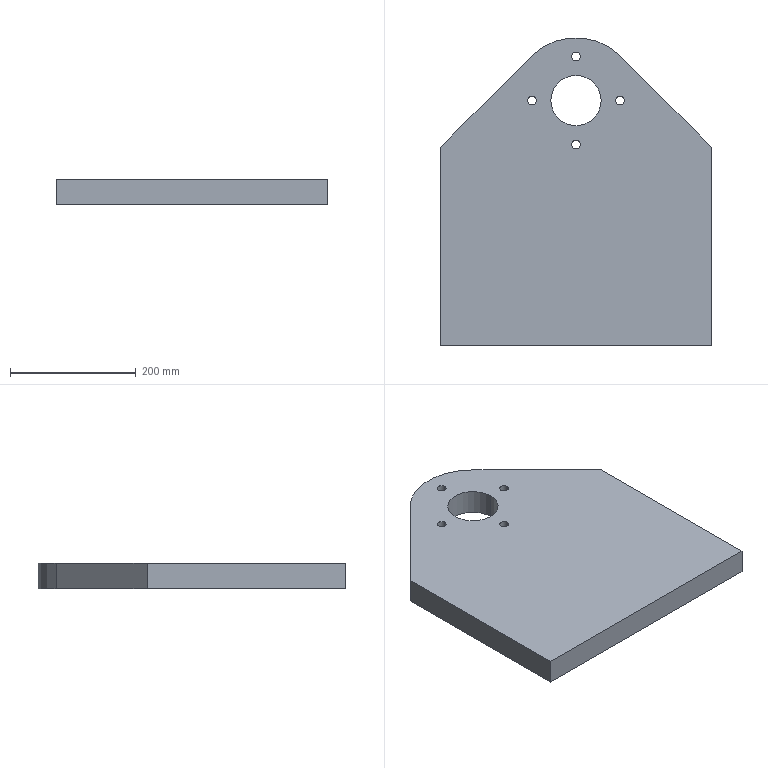Part | SolidWorks | features Extrusion 1, HoleWzd 1 | 1 solid | 18 faces | box 430.2 x 490 x 40 mm | volume 6980590 mm3 | cylinder 11 | plane 7 | commonest cylinder face diameters 14 x8 80 x2 200 x1
STEP:
#1=CARTESIAN_POINT('',(208.1,460.,0.));
#2=VERTEX_POINT('',#1);
#3=CARTESIAN_POINT('',(222.1,460.,0.));
#4=VERTEX_POINT('',#3);
#5=CARTESIAN_POINT('',(215.1,460.,0.));
#6=DIRECTION('',(0.,0.,1.));
#7=DIRECTION('',(1.,0.,0.));
#8=AXIS2_PLACEMENT_3D('',#5,#6,#7);
#9=CIRCLE('',#8,7.);
#10=EDGE_CURVE('',#2,#4,#9,.T.);
#11=ORIENTED_EDGE('',*,*,#10,.F.);
#12=CARTESIAN_POINT('',(208.1,460.,40.));
#13=VERTEX_POINT('',#12);
#14=CARTESIAN_POINT('',(208.1,460.,40.));
#15=DIRECTION('',(0.,0.,1.));
#16=VECTOR('',#15,1000.);
#17=LINE('',#14,#16);
#18=EDGE_CURVE('',#2,#13,#17,.T.);
#19=ORIENTED_EDGE('',*,*,#18,.T.);
#20=CARTESIAN_POINT('',(222.1,460.,40.));
#21=VERTEX_POINT('',#20);
#22=CARTESIAN_POINT('',(215.1,460.,40.));
#23=DIRECTION('',(0.,0.,1.));
#24=DIRECTION('',(1.,0.,0.));
#25=AXIS2_PLACEMENT_3D('',#22,#23,#24);
#26=CIRCLE('',#25,7.);
#27=EDGE_CURVE('',#13,#21,#26,.T.);
#28=ORIENTED_EDGE('',*,*,#27,.T.);
#29=CARTESIAN_POINT('',(222.1,460.,40.));
#30=DIRECTION('',(0.,0.,1.));
#31=VECTOR('',#30,1000.);
#32=LINE('',#29,#31);
#33=EDGE_CURVE('',#4,#21,#32,.T.);
#34=ORIENTED_EDGE('',*,*,#33,.F.);
#35=EDGE_LOOP('',(#11,#19,#28,#34));
#36=FACE_OUTER_BOUND('',#35,.T.);
#37=CARTESIAN_POINT('',(215.1,460.,40.));
#38=DIRECTION('',(0.,0.,1.));
#39=DIRECTION('',(1.,0.,0.));
#40=AXIS2_PLACEMENT_3D('',#37,#38,#39);
#41=CYLINDRICAL_SURFACE('',#40,7.);
#42=ADVANCED_FACE('',(#36),#41,.F.);
#43=CARTESIAN_POINT('',(278.1,390.,0.));
#44=VERTEX_POINT('',#43);
#45=CARTESIAN_POINT('',(292.1,390.,0.));
#46=VERTEX_POINT('',#45);
#47=CARTESIAN_POINT('',(285.1,390.,0.));
#48=DIRECTION('',(0.,0.,1.));
#49=DIRECTION('',(1.,0.,0.));
#50=AXIS2_PLACEMENT_3D('',#47,#48,#49);
#51=CIRCLE('',#50,7.);
#52=EDGE_CURVE('',#44,#46,#51,.T.);
#53=ORIENTED_EDGE('',*,*,#52,.F.);
#54=CARTESIAN_POINT('',(278.1,390.,40.));
#55=VERTEX_POINT('',#54);
#56=CARTESIAN_POINT('',(278.1,390.,40.));
#57=DIRECTION('',(0.,0.,1.));
#58=VECTOR('',#57,1000.);
#59=LINE('',#56,#58);
#60=EDGE_CURVE('',#44,#55,#59,.T.);
#61=ORIENTED_EDGE('',*,*,#60,.T.);
#62=CARTESIAN_POINT('',(292.1,390.,40.));
#63=VERTEX_POINT('',#62);
#64=CARTESIAN_POINT('',(285.1,390.,40.));
#65=DIRECTION('',(0.,0.,1.));
#66=DIRECTION('',(1.,0.,0.));
#67=AXIS2_PLACEMENT_3D('',#64,#65,#66);
#68=CIRCLE('',#67,7.);
#69=EDGE_CURVE('',#55,#63,#68,.T.);
#70=ORIENTED_EDGE('',*,*,#69,.T.);
#71=CARTESIAN_POINT('',(292.1,390.,40.));
#72=DIRECTION('',(0.,0.,1.));
#73=VECTOR('',#72,1000.);
#74=LINE('',#71,#73);
#75=EDGE_CURVE('',#46,#63,#74,.T.);
#76=ORIENTED_EDGE('',*,*,#75,.F.);
#77=EDGE_LOOP('',(#53,#61,#70,#76));
#78=FACE_OUTER_BOUND('',#77,.T.);
#79=CARTESIAN_POINT('',(285.1,390.,40.));
#80=DIRECTION('',(0.,0.,1.));
#81=DIRECTION('',(1.,0.,0.));
#82=AXIS2_PLACEMENT_3D('',#79,#80,#81);
#83=CYLINDRICAL_SURFACE('',#82,7.);
#84=ADVANCED_FACE('',(#78),#83,.F.);
#85=CARTESIAN_POINT('',(208.1,320.,0.));
#86=VERTEX_POINT('',#85);
#87=CARTESIAN_POINT('',(222.1,320.,0.));
#88=VERTEX_POINT('',#87);
#89=CARTESIAN_POINT('',(215.1,320.,0.));
#90=DIRECTION('',(0.,0.,1.));
#91=DIRECTION('',(1.,0.,0.));
#92=AXIS2_PLACEMENT_3D('',#89,#90,#91);
#93=CIRCLE('',#92,7.);
#94=EDGE_CURVE('',#86,#88,#93,.T.);
#95=ORIENTED_EDGE('',*,*,#94,.F.);
#96=CARTESIAN_POINT('',(208.1,320.,40.));
#97=VERTEX_POINT('',#96);
#98=CARTESIAN_POINT('',(208.1,320.,40.));
#99=DIRECTION('',(0.,0.,1.));
#100=VECTOR('',#99,1000.);
#101=LINE('',#98,#100);
#102=EDGE_CURVE('',#86,#97,#101,.T.);
#103=ORIENTED_EDGE('',*,*,#102,.T.);
#104=CARTESIAN_POINT('',(222.1,320.,40.));
#105=VERTEX_POINT('',#104);
#106=CARTESIAN_POINT('',(215.1,320.,40.));
#107=DIRECTION('',(0.,0.,1.));
#108=DIRECTION('',(1.,0.,0.));
#109=AXIS2_PLACEMENT_3D('',#106,#107,#108);
#110=CIRCLE('',#109,7.);
#111=EDGE_CURVE('',#97,#105,#110,.T.);
#112=ORIENTED_EDGE('',*,*,#111,.T.);
#113=CARTESIAN_POINT('',(222.1,320.,40.));
#114=DIRECTION('',(0.,0.,1.));
#115=VECTOR('',#114,1000.);
#116=LINE('',#113,#115);
#117=EDGE_CURVE('',#88,#105,#116,.T.);
#118=ORIENTED_EDGE('',*,*,#117,.F.);
#119=EDGE_LOOP('',(#95,#103,#112,#118));
#120=FACE_OUTER_BOUND('',#119,.T.);
#121=CARTESIAN_POINT('',(215.1,320.,40.));
#122=DIRECTION('',(0.,0.,1.));
#123=DIRECTION('',(1.,0.,0.));
#124=AXIS2_PLACEMENT_3D('',#121,#122,#123);
#125=CYLINDRICAL_SURFACE('',#124,7.);
#126=ADVANCED_FACE('',(#120),#125,.F.);
#127=CARTESIAN_POINT('',(138.1,390.,0.));
#128=VERTEX_POINT('',#127);
#129=CARTESIAN_POINT('',(152.1,390.,0.));
#130=VERTEX_POINT('',#129);
#131=CARTESIAN_POINT('',(145.1,390.,0.));
#132=DIRECTION('',(0.,0.,1.));
#133=DIRECTION('',(1.,0.,0.));
#134=AXIS2_PLACEMENT_3D('',#131,#132,#133);
#135=CIRCLE('',#134,7.);
#136=EDGE_CURVE('',#128,#130,#135,.T.);
#137=ORIENTED_EDGE('',*,*,#136,.F.);
#138=CARTESIAN_POINT('',(138.1,390.,40.));
#139=VERTEX_POINT('',#138);
#140=CARTESIAN_POINT('',(138.1,390.,40.));
#141=DIRECTION('',(0.,0.,1.));
#142=VECTOR('',#141,1000.);
#143=LINE('',#140,#142);
#144=EDGE_CURVE('',#128,#139,#143,.T.);
#145=ORIENTED_EDGE('',*,*,#144,.T.);
#146=CARTESIAN_POINT('',(152.1,390.,40.));
#147=VERTEX_POINT('',#146);
#148=CARTESIAN_POINT('',(145.1,390.,40.));
#149=DIRECTION('',(0.,0.,1.));
#150=DIRECTION('',(1.,0.,0.));
#151=AXIS2_PLACEMENT_3D('',#148,#149,#150);
#152=CIRCLE('',#151,7.);
#153=EDGE_CURVE('',#139,#147,#152,.T.);
#154=ORIENTED_EDGE('',*,*,#153,.T.);
#155=CARTESIAN_POINT('',(152.1,390.,40.));
#156=DIRECTION('',(0.,0.,1.));
#157=VECTOR('',#156,1000.);
#158=LINE('',#155,#157);
#159=EDGE_CURVE('',#130,#147,#158,.T.);
#160=ORIENTED_EDGE('',*,*,#159,.F.);
#161=EDGE_LOOP('',(#137,#145,#154,#160));
#162=FACE_OUTER_BOUND('',#161,.T.);
#163=CARTESIAN_POINT('',(145.1,390.,40.));
#164=DIRECTION('',(0.,0.,1.));
#165=DIRECTION('',(1.,0.,0.));
#166=AXIS2_PLACEMENT_3D('',#163,#164,#165);
#167=CYLINDRICAL_SURFACE('',#166,7.);
#168=ADVANCED_FACE('',(#162),#167,.F.);
#169=CARTESIAN_POINT('',(175.1,390.,40.));
#170=VERTEX_POINT('',#169);
#171=CARTESIAN_POINT('',(255.1,390.,40.));
#172=VERTEX_POINT('',#171);
#173=CARTESIAN_POINT('',(215.1,390.,40.));
#174=DIRECTION('',(0.,0.,1.));
#175=DIRECTION('',(1.,0.,0.));
#176=AXIS2_PLACEMENT_3D('',#173,#174,#175);
#177=CIRCLE('',#176,40.);
#178=EDGE_CURVE('',#170,#172,#177,.T.);
#179=ORIENTED_EDGE('',*,*,#178,.T.);
#180=CARTESIAN_POINT('',(255.1,390.,0.));
#181=VERTEX_POINT('',#180);
#182=CARTESIAN_POINT('',(255.1,390.,40.));
#183=DIRECTION('',(0.,0.,-1.));
#184=VECTOR('',#183,1000.);
#185=LINE('',#182,#184);
#186=EDGE_CURVE('',#172,#181,#185,.T.);
#187=ORIENTED_EDGE('',*,*,#186,.T.);
#188=CARTESIAN_POINT('',(175.1,390.,0.));
#189=VERTEX_POINT('',#188);
#190=CARTESIAN_POINT('',(215.1,390.,0.));
#191=DIRECTION('',(0.,0.,1.));
#192=DIRECTION('',(1.,0.,0.));
#193=AXIS2_PLACEMENT_3D('',#190,#191,#192);
#194=CIRCLE('',#193,40.);
#195=EDGE_CURVE('',#189,#181,#194,.T.);
#196=ORIENTED_EDGE('',*,*,#195,.F.);
#197=CARTESIAN_POINT('',(175.1,390.,40.));
#198=DIRECTION('',(0.,0.,-1.));
#199=VECTOR('',#198,1000.);
#200=LINE('',#197,#199);
#201=EDGE_CURVE('',#170,#189,#200,.T.);
#202=ORIENTED_EDGE('',*,*,#201,.F.);
#203=EDGE_LOOP('',(#179,#187,#196,#202));
#204=FACE_OUTER_BOUND('',#203,.T.);
#205=CARTESIAN_POINT('',(215.1,390.,40.));
#206=DIRECTION('',(0.,0.,-1.));
#207=DIRECTION('',(-1.,0.,0.));
#208=AXIS2_PLACEMENT_3D('',#205,#206,#207);
#209=CYLINDRICAL_SURFACE('',#208,40.);
#210=ADVANCED_FACE('',(#204),#209,.F.);
#211=CARTESIAN_POINT('',(215.1,460.,40.));
#212=DIRECTION('',(0.,0.,1.));
#213=DIRECTION('',(1.,0.,0.));
#214=AXIS2_PLACEMENT_3D('',#211,#212,#213);
#215=CIRCLE('',#214,7.);
#216=EDGE_CURVE('',#21,#13,#215,.T.);
#217=ORIENTED_EDGE('',*,*,#216,.F.);
#218=ORIENTED_EDGE('',*,*,#27,.F.);
#219=EDGE_LOOP('',(#217,#218));
#220=FACE_BOUND('',#219,.T.);
#221=CARTESIAN_POINT('',(285.1,390.,40.));
#222=DIRECTION('',(0.,0.,1.));
#223=DIRECTION('',(1.,0.,0.));
#224=AXIS2_PLACEMENT_3D('',#221,#222,#223);
#225=CIRCLE('',#224,7.);
#226=EDGE_CURVE('',#63,#55,#225,.T.);
#227=ORIENTED_EDGE('',*,*,#226,.F.);
#228=ORIENTED_EDGE('',*,*,#69,.F.);
#229=EDGE_LOOP('',(#227,#228));
#230=FACE_BOUND('',#229,.T.);
#231=CARTESIAN_POINT('',(215.1,320.,40.));
#232=DIRECTION('',(0.,0.,1.));
#233=DIRECTION('',(1.,0.,0.));
#234=AXIS2_PLACEMENT_3D('',#231,#232,#233);
#235=CIRCLE('',#234,7.);
#236=EDGE_CURVE('',#105,#97,#235,.T.);
#237=ORIENTED_EDGE('',*,*,#236,.F.);
#238=ORIENTED_EDGE('',*,*,#111,.F.);
#239=EDGE_LOOP('',(#237,#238));
#240=FACE_BOUND('',#239,.T.);
#241=CARTESIAN_POINT('',(145.1,390.,40.));
#242=DIRECTION('',(0.,0.,1.));
#243=DIRECTION('',(1.,0.,0.));
#244=AXIS2_PLACEMENT_3D('',#241,#242,#243);
#245=CIRCLE('',#244,7.);
#246=EDGE_CURVE('',#147,#139,#245,.T.);
#247=ORIENTED_EDGE('',*,*,#246,.F.);
#248=ORIENTED_EDGE('',*,*,#153,.F.);
#249=EDGE_LOOP('',(#247,#248));
#250=FACE_BOUND('',#249,.T.);
#251=CARTESIAN_POINT('',(0.,316.,40.));
#252=VERTEX_POINT('',#251);
#253=CARTESIAN_POINT('',(0.,0.,40.));
#254=VERTEX_POINT('',#253);
#255=CARTESIAN_POINT('',(0.,0.,40.));
#256=DIRECTION('',(0.,-1.,0.));
#257=VECTOR('',#256,1000.);
#258=LINE('',#255,#257);
#259=EDGE_CURVE('',#252,#254,#258,.T.);
#260=ORIENTED_EDGE('',*,*,#259,.T.);
#261=CARTESIAN_POINT('',(430.2,0.,40.));
#262=VERTEX_POINT('',#261);
#263=CARTESIAN_POINT('',(0.,0.,40.));
#264=DIRECTION('',(1.,0.,0.));
#265=VECTOR('',#264,1000.);
#266=LINE('',#263,#265);
#267=EDGE_CURVE('',#254,#262,#266,.T.);
#268=ORIENTED_EDGE('',*,*,#267,.T.);
#269=CARTESIAN_POINT('',(430.2,316.,40.));
#270=VERTEX_POINT('',#269);
#271=CARTESIAN_POINT('',(430.2,0.,40.));
#272=DIRECTION('',(0.,1.,0.));
#273=VECTOR('',#272,1000.);
#274=LINE('',#271,#273);
#275=EDGE_CURVE('',#262,#270,#274,.T.);
#276=ORIENTED_EDGE('',*,*,#275,.T.);
#277=CARTESIAN_POINT('',(285.889,460.632,40.));
#278=VERTEX_POINT('',#277);
#279=CARTESIAN_POINT('',(430.2,316.,40.));
#280=DIRECTION('',(-0.7063,0.7079,0.));
#281=VECTOR('',#280,1000.);
#282=LINE('',#279,#281);
#283=EDGE_CURVE('',#270,#278,#282,.T.);
#284=ORIENTED_EDGE('',*,*,#283,.T.);
#285=CARTESIAN_POINT('',(144.311,460.632,40.));
#286=VERTEX_POINT('',#285);
#287=CARTESIAN_POINT('',(215.1,390.,40.));
#288=DIRECTION('',(0.,0.,1.));
#289=DIRECTION('',(1.,0.,0.));
#290=AXIS2_PLACEMENT_3D('',#287,#288,#289);
#291=CIRCLE('',#290,100.);
#292=EDGE_CURVE('',#278,#286,#291,.T.);
#293=ORIENTED_EDGE('',*,*,#292,.T.);
#294=CARTESIAN_POINT('',(0.,316.,40.));
#295=DIRECTION('',(-0.7063,-0.7079,0.));
#296=VECTOR('',#295,1000.);
#297=LINE('',#294,#296);
#298=EDGE_CURVE('',#286,#252,#297,.T.);
#299=ORIENTED_EDGE('',*,*,#298,.T.);
#300=EDGE_LOOP('',(#260,#268,#276,#284,#293,#299));
#301=FACE_OUTER_BOUND('',#300,.T.);
#302=ORIENTED_EDGE('',*,*,#178,.F.);
#303=CARTESIAN_POINT('',(215.1,390.,40.));
#304=DIRECTION('',(0.,0.,1.));
#305=DIRECTION('',(1.,0.,0.));
#306=AXIS2_PLACEMENT_3D('',#303,#304,#305);
#307=CIRCLE('',#306,40.);
#308=EDGE_CURVE('',#172,#170,#307,.T.);
#309=ORIENTED_EDGE('',*,*,#308,.F.);
#310=EDGE_LOOP('',(#302,#309));
#311=FACE_BOUND('',#310,.T.);
#312=CARTESIAN_POINT('',(215.1,390.,40.));
#313=DIRECTION('',(0.,0.,1.));
#314=DIRECTION('',(1.,0.,0.));
#315=AXIS2_PLACEMENT_3D('',#312,#313,#314);
#316=PLANE('',#315);
#317=ADVANCED_FACE('',(#220,#230,#240,#250,#301,#311),#316,.T.);
#318=CARTESIAN_POINT('',(215.1,460.,0.));
#319=DIRECTION('',(0.,0.,1.));
#320=DIRECTION('',(1.,0.,0.));
#321=AXIS2_PLACEMENT_3D('',#318,#319,#320);
#322=CIRCLE('',#321,7.);
#323=EDGE_CURVE('',#4,#2,#322,.T.);
#324=ORIENTED_EDGE('',*,*,#323,.T.);
#325=ORIENTED_EDGE('',*,*,#10,.T.);
#326=EDGE_LOOP('',(#324,#325));
#327=FACE_BOUND('',#326,.T.);
#328=CARTESIAN_POINT('',(285.1,390.,0.));
#329=DIRECTION('',(0.,0.,1.));
#330=DIRECTION('',(1.,0.,0.));
#331=AXIS2_PLACEMENT_3D('',#328,#329,#330);
#332=CIRCLE('',#331,7.);
#333=EDGE_CURVE('',#46,#44,#332,.T.);
#334=ORIENTED_EDGE('',*,*,#333,.T.);
#335=ORIENTED_EDGE('',*,*,#52,.T.);
#336=EDGE_LOOP('',(#334,#335));
#337=FACE_BOUND('',#336,.T.);
#338=CARTESIAN_POINT('',(215.1,320.,0.));
#339=DIRECTION('',(0.,0.,1.));
#340=DIRECTION('',(1.,0.,0.));
#341=AXIS2_PLACEMENT_3D('',#338,#339,#340);
#342=CIRCLE('',#341,7.);
#343=EDGE_CURVE('',#88,#86,#342,.T.);
#344=ORIENTED_EDGE('',*,*,#343,.T.);
#345=ORIENTED_EDGE('',*,*,#94,.T.);
#346=EDGE_LOOP('',(#344,#345));
#347=FACE_BOUND('',#346,.T.);
#348=CARTESIAN_POINT('',(145.1,390.,0.));
#349=DIRECTION('',(0.,0.,1.));
#350=DIRECTION('',(1.,0.,0.));
#351=AXIS2_PLACEMENT_3D('',#348,#349,#350);
#352=CIRCLE('',#351,7.);
#353=EDGE_CURVE('',#130,#128,#352,.T.);
#354=ORIENTED_EDGE('',*,*,#353,.T.);
#355=ORIENTED_EDGE('',*,*,#136,.T.);
#356=EDGE_LOOP('',(#354,#355));
#357=FACE_BOUND('',#356,.T.);
#358=CARTESIAN_POINT('',(0.,316.,0.));
#359=VERTEX_POINT('',#358);
#360=CARTESIAN_POINT('',(0.,0.,0.));
#361=VERTEX_POINT('',#360);
#362=CARTESIAN_POINT('',(0.,0.,0.));
#363=DIRECTION('',(0.,-1.,0.));
#364=VECTOR('',#363,1000.);
#365=LINE('',#362,#364);
#366=EDGE_CURVE('',#359,#361,#365,.T.);
#367=ORIENTED_EDGE('',*,*,#366,.F.);
#368=CARTESIAN_POINT('',(144.311,460.632,0.));
#369=VERTEX_POINT('',#368);
#370=CARTESIAN_POINT('',(0.,316.,0.));
#371=DIRECTION('',(-0.7063,-0.7079,0.));
#372=VECTOR('',#371,1000.);
#373=LINE('',#370,#372);
#374=EDGE_CURVE('',#369,#359,#373,.T.);
#375=ORIENTED_EDGE('',*,*,#374,.F.);
#376=CARTESIAN_POINT('',(285.889,460.632,0.));
#377=VERTEX_POINT('',#376);
#378=CARTESIAN_POINT('',(215.1,390.,0.));
#379=DIRECTION('',(0.,0.,1.));
#380=DIRECTION('',(1.,0.,0.));
#381=AXIS2_PLACEMENT_3D('',#378,#379,#380);
#382=CIRCLE('',#381,100.);
#383=EDGE_CURVE('',#377,#369,#382,.T.);
#384=ORIENTED_EDGE('',*,*,#383,.F.);
#385=CARTESIAN_POINT('',(430.2,316.,0.));
#386=VERTEX_POINT('',#385);
#387=CARTESIAN_POINT('',(430.2,316.,0.));
#388=DIRECTION('',(-0.7063,0.7079,0.));
#389=VECTOR('',#388,1000.);
#390=LINE('',#387,#389);
#391=EDGE_CURVE('',#386,#377,#390,.T.);
#392=ORIENTED_EDGE('',*,*,#391,.F.);
#393=CARTESIAN_POINT('',(430.2,0.,0.));
#394=VERTEX_POINT('',#393);
#395=CARTESIAN_POINT('',(430.2,0.,0.));
#396=DIRECTION('',(0.,1.,0.));
#397=VECTOR('',#396,1000.);
#398=LINE('',#395,#397);
#399=EDGE_CURVE('',#394,#386,#398,.T.);
#400=ORIENTED_EDGE('',*,*,#399,.F.);
#401=CARTESIAN_POINT('',(0.,0.,0.));
#402=DIRECTION('',(1.,0.,0.));
#403=VECTOR('',#402,1000.);
#404=LINE('',#401,#403);
#405=EDGE_CURVE('',#361,#394,#404,.T.);
#406=ORIENTED_EDGE('',*,*,#405,.F.);
#407=EDGE_LOOP('',(#367,#375,#384,#392,#400,#406));
#408=FACE_OUTER_BOUND('',#407,.T.);
#409=ORIENTED_EDGE('',*,*,#195,.T.);
#410=CARTESIAN_POINT('',(215.1,390.,0.));
#411=DIRECTION('',(0.,0.,1.));
#412=DIRECTION('',(1.,0.,0.));
#413=AXIS2_PLACEMENT_3D('',#410,#411,#412);
#414=CIRCLE('',#413,40.);
#415=EDGE_CURVE('',#181,#189,#414,.T.);
#416=ORIENTED_EDGE('',*,*,#415,.T.);
#417=EDGE_LOOP('',(#409,#416));
#418=FACE_BOUND('',#417,.T.);
#419=CARTESIAN_POINT('',(215.1,390.,0.));
#420=DIRECTION('',(0.,0.,1.));
#421=DIRECTION('',(1.,0.,0.));
#422=AXIS2_PLACEMENT_3D('',#419,#420,#421);
#423=PLANE('',#422);
#424=ADVANCED_FACE('',(#327,#337,#347,#357,#408,#418),#423,.F.);
#425=ORIENTED_EDGE('',*,*,#366,.T.);
#426=CARTESIAN_POINT('',(0.,0.,40.));
#427=DIRECTION('',(0.,0.,-1.));
#428=VECTOR('',#427,1000.);
#429=LINE('',#426,#428);
#430=EDGE_CURVE('',#254,#361,#429,.T.);
#431=ORIENTED_EDGE('',*,*,#430,.F.);
#432=ORIENTED_EDGE('',*,*,#259,.F.);
#433=CARTESIAN_POINT('',(0.,316.,40.));
#434=DIRECTION('',(0.,0.,-1.));
#435=VECTOR('',#434,1000.);
#436=LINE('',#433,#435);
#437=EDGE_CURVE('',#252,#359,#436,.T.);
#438=ORIENTED_EDGE('',*,*,#437,.T.);
#439=EDGE_LOOP('',(#425,#431,#432,#438));
#440=FACE_OUTER_BOUND('',#439,.T.);
#441=CARTESIAN_POINT('',(0.,0.,40.));
#442=DIRECTION('',(1.,0.,0.));
#443=DIRECTION('',(0.,0.,-1.));
#444=AXIS2_PLACEMENT_3D('',#441,#442,#443);
#445=PLANE('',#444);
#446=ADVANCED_FACE('',(#440),#445,.F.);
#447=ORIENTED_EDGE('',*,*,#405,.T.);
#448=CARTESIAN_POINT('',(430.2,0.,40.));
#449=DIRECTION('',(0.,0.,-1.));
#450=VECTOR('',#449,1000.);
#451=LINE('',#448,#450);
#452=EDGE_CURVE('',#262,#394,#451,.T.);
#453=ORIENTED_EDGE('',*,*,#452,.F.);
#454=ORIENTED_EDGE('',*,*,#267,.F.);
#455=ORIENTED_EDGE('',*,*,#430,.T.);
#456=EDGE_LOOP('',(#447,#453,#454,#455));
#457=FACE_OUTER_BOUND('',#456,.T.);
#458=CARTESIAN_POINT('',(0.,0.,40.));
#459=DIRECTION('',(0.,1.,0.));
#460=DIRECTION('',(0.,0.,1.));
#461=AXIS2_PLACEMENT_3D('',#458,#459,#460);
#462=PLANE('',#461);
#463=ADVANCED_FACE('',(#457),#462,.F.);
#464=ORIENTED_EDGE('',*,*,#399,.T.);
#465=CARTESIAN_POINT('',(430.2,316.,40.));
#466=DIRECTION('',(0.,0.,-1.));
#467=VECTOR('',#466,1000.);
#468=LINE('',#465,#467);
#469=EDGE_CURVE('',#270,#386,#468,.T.);
#470=ORIENTED_EDGE('',*,*,#469,.F.);
#471=ORIENTED_EDGE('',*,*,#275,.F.);
#472=ORIENTED_EDGE('',*,*,#452,.T.);
#473=EDGE_LOOP('',(#464,#470,#471,#472));
#474=FACE_OUTER_BOUND('',#473,.T.);
#475=CARTESIAN_POINT('',(430.2,0.,40.));
#476=DIRECTION('',(-1.,0.,0.));
#477=DIRECTION('',(0.,0.,1.));
#478=AXIS2_PLACEMENT_3D('',#475,#476,#477);
#479=PLANE('',#478);
#480=ADVANCED_FACE('',(#474),#479,.F.);
#481=ORIENTED_EDGE('',*,*,#391,.T.);
#482=CARTESIAN_POINT('',(285.889,460.632,40.));
#483=DIRECTION('',(0.,0.,-1.));
#484=VECTOR('',#483,1000.);
#485=LINE('',#482,#484);
#486=EDGE_CURVE('',#278,#377,#485,.T.);
#487=ORIENTED_EDGE('',*,*,#486,.F.);
#488=ORIENTED_EDGE('',*,*,#283,.F.);
#489=ORIENTED_EDGE('',*,*,#469,.T.);
#490=EDGE_LOOP('',(#481,#487,#488,#489));
#491=FACE_OUTER_BOUND('',#490,.T.);
#492=CARTESIAN_POINT('',(430.2,316.,40.));
#493=DIRECTION('',(-0.7079,-0.7063,0.));
#494=DIRECTION('',(0.7063,-0.7079,0.));
#495=AXIS2_PLACEMENT_3D('',#492,#493,#494);
#496=PLANE('',#495);
#497=ADVANCED_FACE('',(#491),#496,.F.);
#498=ORIENTED_EDGE('',*,*,#383,.T.);
#499=CARTESIAN_POINT('',(144.311,460.632,40.));
#500=DIRECTION('',(0.,0.,-1.));
#501=VECTOR('',#500,1000.);
#502=LINE('',#499,#501);
#503=EDGE_CURVE('',#286,#369,#502,.T.);
#504=ORIENTED_EDGE('',*,*,#503,.F.);
#505=ORIENTED_EDGE('',*,*,#292,.F.);
#506=ORIENTED_EDGE('',*,*,#486,.T.);
#507=EDGE_LOOP('',(#498,#504,#505,#506));
#508=FACE_OUTER_BOUND('',#507,.T.);
#509=CARTESIAN_POINT('',(215.1,390.,40.));
#510=DIRECTION('',(0.,0.,-1.));
#511=DIRECTION('',(-1.,0.,0.));
#512=AXIS2_PLACEMENT_3D('',#509,#510,#511);
#513=CYLINDRICAL_SURFACE('',#512,100.);
#514=ADVANCED_FACE('',(#508),#513,.T.);
#515=ORIENTED_EDGE('',*,*,#374,.T.);
#516=ORIENTED_EDGE('',*,*,#437,.F.);
#517=ORIENTED_EDGE('',*,*,#298,.F.);
#518=ORIENTED_EDGE('',*,*,#503,.T.);
#519=EDGE_LOOP('',(#515,#516,#517,#518));
#520=FACE_OUTER_BOUND('',#519,.T.);
#521=CARTESIAN_POINT('',(0.,316.,40.));
#522=DIRECTION('',(0.7079,-0.7063,0.));
#523=DIRECTION('',(0.7063,0.7079,0.));
#524=AXIS2_PLACEMENT_3D('',#521,#522,#523);
#525=PLANE('',#524);
#526=ADVANCED_FACE('',(#520),#525,.F.);
#527=ORIENTED_EDGE('',*,*,#186,.F.);
#528=ORIENTED_EDGE('',*,*,#308,.T.);
#529=ORIENTED_EDGE('',*,*,#201,.T.);
#530=ORIENTED_EDGE('',*,*,#415,.F.);
#531=EDGE_LOOP('',(#527,#528,#529,#530));
#532=FACE_OUTER_BOUND('',#531,.T.);
#533=CARTESIAN_POINT('',(215.1,390.,40.));
#534=DIRECTION('',(0.,0.,-1.));
#535=DIRECTION('',(-1.,0.,0.));
#536=AXIS2_PLACEMENT_3D('',#533,#534,#535);
#537=CYLINDRICAL_SURFACE('',#536,40.);
#538=ADVANCED_FACE('',(#532),#537,.F.);
#539=ORIENTED_EDGE('',*,*,#144,.F.);
#540=ORIENTED_EDGE('',*,*,#353,.F.);
#541=ORIENTED_EDGE('',*,*,#159,.T.);
#542=ORIENTED_EDGE('',*,*,#246,.T.);
#543=EDGE_LOOP('',(#539,#540,#541,#542));
#544=FACE_OUTER_BOUND('',#543,.T.);
#545=CARTESIAN_POINT('',(145.1,390.,40.));
#546=DIRECTION('',(0.,0.,1.));
#547=DIRECTION('',(1.,0.,0.));
#548=AXIS2_PLACEMENT_3D('',#545,#546,#547);
#549=CYLINDRICAL_SURFACE('',#548,7.);
#550=ADVANCED_FACE('',(#544),#549,.F.);
#551=ORIENTED_EDGE('',*,*,#102,.F.);
#552=ORIENTED_EDGE('',*,*,#343,.F.);
#553=ORIENTED_EDGE('',*,*,#117,.T.);
#554=ORIENTED_EDGE('',*,*,#236,.T.);
#555=EDGE_LOOP('',(#551,#552,#553,#554));
#556=FACE_OUTER_BOUND('',#555,.T.);
#557=CARTESIAN_POINT('',(215.1,320.,40.));
#558=DIRECTION('',(0.,0.,1.));
#559=DIRECTION('',(1.,0.,0.));
#560=AXIS2_PLACEMENT_3D('',#557,#558,#559);
#561=CYLINDRICAL_SURFACE('',#560,7.);
#562=ADVANCED_FACE('',(#556),#561,.F.);
#563=ORIENTED_EDGE('',*,*,#60,.F.);
#564=ORIENTED_EDGE('',*,*,#333,.F.);
#565=ORIENTED_EDGE('',*,*,#75,.T.);
#566=ORIENTED_EDGE('',*,*,#226,.T.);
#567=EDGE_LOOP('',(#563,#564,#565,#566));
#568=FACE_OUTER_BOUND('',#567,.T.);
#569=CARTESIAN_POINT('',(285.1,390.,40.));
#570=DIRECTION('',(0.,0.,1.));
#571=DIRECTION('',(1.,0.,0.));
#572=AXIS2_PLACEMENT_3D('',#569,#570,#571);
#573=CYLINDRICAL_SURFACE('',#572,7.);
#574=ADVANCED_FACE('',(#568),#573,.F.);
#575=ORIENTED_EDGE('',*,*,#18,.F.);
#576=ORIENTED_EDGE('',*,*,#323,.F.);
#577=ORIENTED_EDGE('',*,*,#33,.T.);
#578=ORIENTED_EDGE('',*,*,#216,.T.);
#579=EDGE_LOOP('',(#575,#576,#577,#578));
#580=FACE_OUTER_BOUND('',#579,.T.);
#581=CARTESIAN_POINT('',(215.1,460.,40.));
#582=DIRECTION('',(0.,0.,1.));
#583=DIRECTION('',(1.,0.,0.));
#584=AXIS2_PLACEMENT_3D('',#581,#582,#583);
#585=CYLINDRICAL_SURFACE('',#584,7.);
#586=ADVANCED_FACE('',(#580),#585,.F.);
#587=CLOSED_SHELL('',(#42,#84,#126,#168,#210,#317,#424,#446,#463,#480,#497,#514,#526,#538,#550,#562,#574,#586));
#588=MANIFOLD_SOLID_BREP('',#587);
#589=CARTESIAN_POINT('',(0.,0.,0.));
#590=DIRECTION('',(0.,0.,1.));
#591=DIRECTION('',(1.,0.,0.));
#592=AXIS2_PLACEMENT_3D('',#589,#590,#591);
#593=(LENGTH_UNIT()NAMED_UNIT(*)SI_UNIT(.MILLI.,.METRE.));
#594=UNCERTAINTY_MEASURE_WITH_UNIT(LENGTH_MEASURE(0.00001),#593,'','');
#595=(NAMED_UNIT(*)PLANE_ANGLE_UNIT()SI_UNIT($,.RADIAN.));
#596=(NAMED_UNIT(*)SI_UNIT($,.STERADIAN.)SOLID_ANGLE_UNIT());
#597=(GEOMETRIC_REPRESENTATION_CONTEXT(3)GLOBAL_UNCERTAINTY_ASSIGNED_CONTEXT((#594))GLOBAL_UNIT_ASSIGNED_CONTEXT((#593,#595,#596))REPRESENTATION_CONTEXT('',''));
#598=ADVANCED_BREP_SHAPE_REPRESENTATION('',(#588,#592),#597);